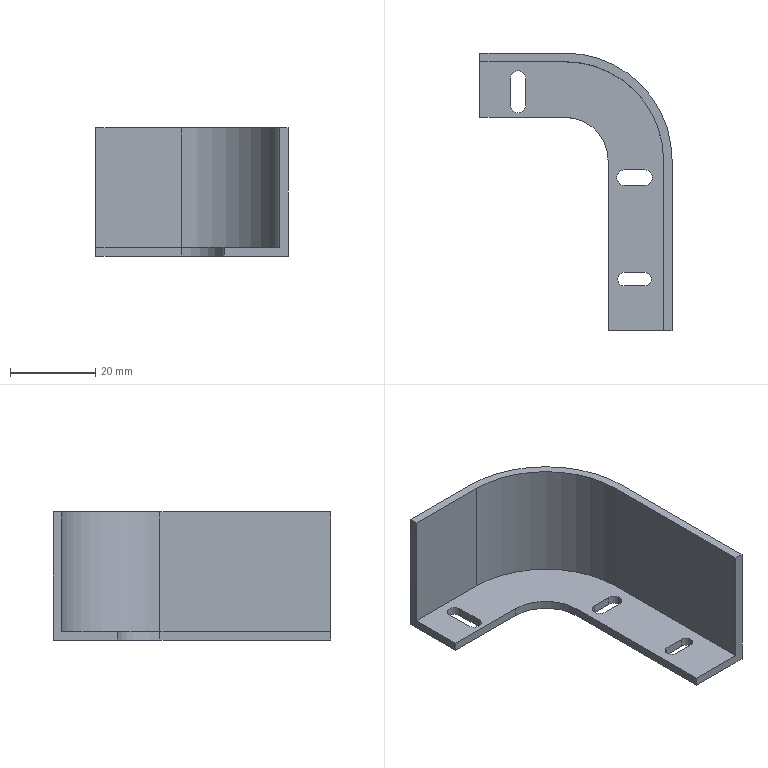Part | SolidWorks | features ICE 2, ExtruThin 1 | 1 solid | 28 faces | box 45 x 65 x 30 mm | volume 7932 mm3 | plane 17 | cylinder 11 | commonest cylinder face diameters 3.152 x3 3.6 x3 3.503 x2 20 x1 46 x1 50 x1
STEP:
#1=CARTESIAN_POINT('',(10.165,12.12,0.));
#2=VERTEX_POINT('',#1);
#3=CARTESIAN_POINT('',(8.588,13.696,0.));
#4=VERTEX_POINT('',#3);
#5=CARTESIAN_POINT('',(8.588,12.12,0.));
#6=DIRECTION('',(0.,0.,1.));
#7=DIRECTION('',(1.,0.,0.));
#8=AXIS2_PLACEMENT_3D('',#5,#6,#7);
#9=CIRCLE('',#8,1.576);
#10=EDGE_CURVE('',#2,#4,#9,.T.);
#11=ORIENTED_EDGE('',*,*,#10,.F.);
#12=CARTESIAN_POINT('',(10.165,12.12,2.));
#13=VERTEX_POINT('',#12);
#14=CARTESIAN_POINT('',(10.165,12.12,-26.));
#15=DIRECTION('',(0.,0.,1.));
#16=VECTOR('',#15,1000.);
#17=LINE('',#14,#16);
#18=EDGE_CURVE('',#2,#13,#17,.T.);
#19=ORIENTED_EDGE('',*,*,#18,.T.);
#20=CARTESIAN_POINT('',(8.588,13.696,2.));
#21=VERTEX_POINT('',#20);
#22=CARTESIAN_POINT('',(8.588,12.12,2.));
#23=DIRECTION('',(0.,0.,1.));
#24=DIRECTION('',(1.,0.,0.));
#25=AXIS2_PLACEMENT_3D('',#22,#23,#24);
#26=CIRCLE('',#25,1.576);
#27=EDGE_CURVE('',#13,#21,#26,.T.);
#28=ORIENTED_EDGE('',*,*,#27,.T.);
#29=CARTESIAN_POINT('',(8.588,13.696,-26.));
#30=DIRECTION('',(0.,0.,1.));
#31=VECTOR('',#30,1000.);
#32=LINE('',#29,#31);
#33=EDGE_CURVE('',#4,#21,#32,.T.);
#34=ORIENTED_EDGE('',*,*,#33,.F.);
#35=EDGE_LOOP('',(#11,#19,#28,#34));
#36=FACE_OUTER_BOUND('',#35,.T.);
#37=CARTESIAN_POINT('',(8.588,12.12,-26.));
#38=DIRECTION('',(0.,0.,1.));
#39=DIRECTION('',(1.,0.,0.));
#40=AXIS2_PLACEMENT_3D('',#37,#38,#39);
#41=CYLINDRICAL_SURFACE('',#40,1.576);
#42=ADVANCED_FACE('',(#36),#41,.F.);
#43=CARTESIAN_POINT('',(10.388,35.907,0.));
#44=VERTEX_POINT('',#43);
#45=CARTESIAN_POINT('',(8.588,37.707,0.));
#46=VERTEX_POINT('',#45);
#47=CARTESIAN_POINT('',(8.588,35.907,0.));
#48=DIRECTION('',(0.,0.,1.));
#49=DIRECTION('',(1.,0.,0.));
#50=AXIS2_PLACEMENT_3D('',#47,#48,#49);
#51=CIRCLE('',#50,1.8);
#52=EDGE_CURVE('',#44,#46,#51,.T.);
#53=ORIENTED_EDGE('',*,*,#52,.F.);
#54=CARTESIAN_POINT('',(10.388,35.907,2.));
#55=VERTEX_POINT('',#54);
#56=CARTESIAN_POINT('',(10.388,35.907,-26.));
#57=DIRECTION('',(0.,0.,1.));
#58=VECTOR('',#57,1000.);
#59=LINE('',#56,#58);
#60=EDGE_CURVE('',#44,#55,#59,.T.);
#61=ORIENTED_EDGE('',*,*,#60,.T.);
#62=CARTESIAN_POINT('',(8.588,37.707,2.));
#63=VERTEX_POINT('',#62);
#64=CARTESIAN_POINT('',(8.588,35.907,2.));
#65=DIRECTION('',(0.,0.,1.));
#66=DIRECTION('',(1.,0.,0.));
#67=AXIS2_PLACEMENT_3D('',#64,#65,#66);
#68=CIRCLE('',#67,1.8);
#69=EDGE_CURVE('',#55,#63,#68,.T.);
#70=ORIENTED_EDGE('',*,*,#69,.T.);
#71=CARTESIAN_POINT('',(8.588,37.707,-26.));
#72=DIRECTION('',(0.,0.,1.));
#73=VECTOR('',#72,1000.);
#74=LINE('',#71,#73);
#75=EDGE_CURVE('',#46,#63,#74,.T.);
#76=ORIENTED_EDGE('',*,*,#75,.F.);
#77=EDGE_LOOP('',(#53,#61,#70,#76));
#78=FACE_OUTER_BOUND('',#77,.T.);
#79=CARTESIAN_POINT('',(8.588,35.907,-26.));
#80=DIRECTION('',(0.,0.,1.));
#81=DIRECTION('',(1.,0.,0.));
#82=AXIS2_PLACEMENT_3D('',#79,#80,#81);
#83=CYLINDRICAL_SURFACE('',#82,1.8);
#84=ADVANCED_FACE('',(#78),#83,.F.);
#85=CARTESIAN_POINT('',(-10.,65.,0.));
#86=VERTEX_POINT('',#85);
#87=CARTESIAN_POINT('',(-30.,65.,0.));
#88=VERTEX_POINT('',#87);
#89=CARTESIAN_POINT('',(-10.,65.,0.));
#90=DIRECTION('',(-1.,0.,0.));
#91=VECTOR('',#90,1000.);
#92=LINE('',#89,#91);
#93=EDGE_CURVE('',#86,#88,#92,.T.);
#94=ORIENTED_EDGE('',*,*,#93,.T.);
#95=CARTESIAN_POINT('',(-30.,65.,30.));
#96=VERTEX_POINT('',#95);
#97=CARTESIAN_POINT('',(-30.,65.,2.));
#98=DIRECTION('',(0.,0.,-1.));
#99=VECTOR('',#98,1000.);
#100=LINE('',#97,#99);
#101=EDGE_CURVE('',#96,#88,#100,.T.);
#102=ORIENTED_EDGE('',*,*,#101,.F.);
#103=CARTESIAN_POINT('',(-10.,65.,30.));
#104=VERTEX_POINT('',#103);
#105=CARTESIAN_POINT('',(-10.,65.,30.));
#106=DIRECTION('',(-1.,0.,0.));
#107=VECTOR('',#106,1000.);
#108=LINE('',#105,#107);
#109=EDGE_CURVE('',#104,#96,#108,.T.);
#110=ORIENTED_EDGE('',*,*,#109,.F.);
#111=CARTESIAN_POINT('',(-10.,65.,2.));
#112=DIRECTION('',(0.,0.,-1.));
#113=VECTOR('',#112,1000.);
#114=LINE('',#111,#113);
#115=EDGE_CURVE('',#104,#86,#114,.T.);
#116=ORIENTED_EDGE('',*,*,#115,.T.);
#117=EDGE_LOOP('',(#94,#102,#110,#116));
#118=FACE_OUTER_BOUND('',#117,.T.);
#119=CARTESIAN_POINT('',(-10.,65.,2.));
#120=DIRECTION('',(0.,-1.,0.));
#121=DIRECTION('',(1.,0.,0.));
#122=AXIS2_PLACEMENT_3D('',#119,#120,#121);
#123=PLANE('',#122);
#124=ADVANCED_FACE('',(#118),#123,.F.);
#125=CARTESIAN_POINT('',(-30.,50.,0.));
#126=VERTEX_POINT('',#125);
#127=CARTESIAN_POINT('',(-30.,50.,0.));
#128=DIRECTION('',(0.,1.,0.));
#129=VECTOR('',#128,1000.);
#130=LINE('',#127,#129);
#131=EDGE_CURVE('',#126,#88,#130,.T.);
#132=ORIENTED_EDGE('',*,*,#131,.F.);
#133=CARTESIAN_POINT('',(-30.,50.,2.));
#134=VERTEX_POINT('',#133);
#135=CARTESIAN_POINT('',(-30.,50.,2.));
#136=DIRECTION('',(0.,0.,-1.));
#137=VECTOR('',#136,1000.);
#138=LINE('',#135,#137);
#139=EDGE_CURVE('',#134,#126,#138,.T.);
#140=ORIENTED_EDGE('',*,*,#139,.F.);
#141=CARTESIAN_POINT('',(-30.,63.,2.));
#142=VERTEX_POINT('',#141);
#143=CARTESIAN_POINT('',(-30.,50.,2.));
#144=DIRECTION('',(0.,1.,0.));
#145=VECTOR('',#144,1000.);
#146=LINE('',#143,#145);
#147=EDGE_CURVE('',#134,#142,#146,.T.);
#148=ORIENTED_EDGE('',*,*,#147,.T.);
#149=CARTESIAN_POINT('',(-30.,63.,30.));
#150=VERTEX_POINT('',#149);
#151=CARTESIAN_POINT('',(-30.,63.,30.));
#152=DIRECTION('',(0.,0.,-1.));
#153=VECTOR('',#152,1000.);
#154=LINE('',#151,#153);
#155=EDGE_CURVE('',#150,#142,#154,.T.);
#156=ORIENTED_EDGE('',*,*,#155,.F.);
#157=CARTESIAN_POINT('',(-30.,65.,30.));
#158=DIRECTION('',(0.,-1.,0.));
#159=VECTOR('',#158,1000.);
#160=LINE('',#157,#159);
#161=EDGE_CURVE('',#96,#150,#160,.T.);
#162=ORIENTED_EDGE('',*,*,#161,.F.);
#163=ORIENTED_EDGE('',*,*,#101,.T.);
#164=EDGE_LOOP('',(#132,#140,#148,#156,#162,#163));
#165=FACE_OUTER_BOUND('',#164,.T.);
#166=CARTESIAN_POINT('',(-30.,50.,2.));
#167=DIRECTION('',(-1.,0.,0.));
#168=DIRECTION('',(0.,-1.,0.));
#169=AXIS2_PLACEMENT_3D('',#166,#167,#168);
#170=PLANE('',#169);
#171=ADVANCED_FACE('',(#165),#170,.T.);
#172=CARTESIAN_POINT('',(-10.,50.,0.));
#173=VERTEX_POINT('',#172);
#174=CARTESIAN_POINT('',(-10.,50.,0.));
#175=DIRECTION('',(-1.,0.,0.));
#176=VECTOR('',#175,1000.);
#177=LINE('',#174,#176);
#178=EDGE_CURVE('',#173,#126,#177,.T.);
#179=ORIENTED_EDGE('',*,*,#178,.F.);
#180=CARTESIAN_POINT('',(-10.,50.,2.));
#181=VERTEX_POINT('',#180);
#182=CARTESIAN_POINT('',(-10.,50.,2.));
#183=DIRECTION('',(0.,0.,-1.));
#184=VECTOR('',#183,1000.);
#185=LINE('',#182,#184);
#186=EDGE_CURVE('',#181,#173,#185,.T.);
#187=ORIENTED_EDGE('',*,*,#186,.F.);
#188=CARTESIAN_POINT('',(-10.,50.,2.));
#189=DIRECTION('',(-1.,0.,0.));
#190=VECTOR('',#189,1000.);
#191=LINE('',#188,#190);
#192=EDGE_CURVE('',#181,#134,#191,.T.);
#193=ORIENTED_EDGE('',*,*,#192,.T.);
#194=ORIENTED_EDGE('',*,*,#139,.T.);
#195=EDGE_LOOP('',(#179,#187,#193,#194));
#196=FACE_OUTER_BOUND('',#195,.T.);
#197=CARTESIAN_POINT('',(-10.,50.,2.));
#198=DIRECTION('',(0.,-1.,0.));
#199=DIRECTION('',(1.,0.,0.));
#200=AXIS2_PLACEMENT_3D('',#197,#198,#199);
#201=PLANE('',#200);
#202=ADVANCED_FACE('',(#196),#201,.T.);
#203=CARTESIAN_POINT('',(0.,40.,0.));
#204=VERTEX_POINT('',#203);
#205=CARTESIAN_POINT('',(-10.,40.,0.));
#206=DIRECTION('',(0.,0.,1.));
#207=DIRECTION('',(1.,0.,0.));
#208=AXIS2_PLACEMENT_3D('',#205,#206,#207);
#209=CIRCLE('',#208,10.);
#210=EDGE_CURVE('',#204,#173,#209,.T.);
#211=ORIENTED_EDGE('',*,*,#210,.F.);
#212=CARTESIAN_POINT('',(0.,40.,2.));
#213=VERTEX_POINT('',#212);
#214=CARTESIAN_POINT('',(0.,40.,2.));
#215=DIRECTION('',(0.,0.,-1.));
#216=VECTOR('',#215,1000.);
#217=LINE('',#214,#216);
#218=EDGE_CURVE('',#213,#204,#217,.T.);
#219=ORIENTED_EDGE('',*,*,#218,.F.);
#220=CARTESIAN_POINT('',(-10.,40.,2.));
#221=DIRECTION('',(0.,0.,1.));
#222=DIRECTION('',(1.,0.,0.));
#223=AXIS2_PLACEMENT_3D('',#220,#221,#222);
#224=CIRCLE('',#223,10.);
#225=EDGE_CURVE('',#213,#181,#224,.T.);
#226=ORIENTED_EDGE('',*,*,#225,.T.);
#227=ORIENTED_EDGE('',*,*,#186,.T.);
#228=EDGE_LOOP('',(#211,#219,#226,#227));
#229=FACE_OUTER_BOUND('',#228,.T.);
#230=CARTESIAN_POINT('',(-10.,40.,2.));
#231=DIRECTION('',(0.,0.,-1.));
#232=DIRECTION('',(-1.,0.,0.));
#233=AXIS2_PLACEMENT_3D('',#230,#231,#232);
#234=CYLINDRICAL_SURFACE('',#233,10.);
#235=ADVANCED_FACE('',(#229),#234,.F.);
#236=CARTESIAN_POINT('',(0.,0.,0.));
#237=VERTEX_POINT('',#236);
#238=CARTESIAN_POINT('',(0.,0.,0.));
#239=DIRECTION('',(0.,1.,0.));
#240=VECTOR('',#239,1000.);
#241=LINE('',#238,#240);
#242=EDGE_CURVE('',#237,#204,#241,.T.);
#243=ORIENTED_EDGE('',*,*,#242,.F.);
#244=CARTESIAN_POINT('',(0.,0.,2.));
#245=VERTEX_POINT('',#244);
#246=CARTESIAN_POINT('',(0.,0.,2.));
#247=DIRECTION('',(0.,0.,-1.));
#248=VECTOR('',#247,1000.);
#249=LINE('',#246,#248);
#250=EDGE_CURVE('',#245,#237,#249,.T.);
#251=ORIENTED_EDGE('',*,*,#250,.F.);
#252=CARTESIAN_POINT('',(0.,0.,2.));
#253=DIRECTION('',(0.,1.,0.));
#254=VECTOR('',#253,1000.);
#255=LINE('',#252,#254);
#256=EDGE_CURVE('',#245,#213,#255,.T.);
#257=ORIENTED_EDGE('',*,*,#256,.T.);
#258=ORIENTED_EDGE('',*,*,#218,.T.);
#259=EDGE_LOOP('',(#243,#251,#257,#258));
#260=FACE_OUTER_BOUND('',#259,.T.);
#261=CARTESIAN_POINT('',(0.,0.,2.));
#262=DIRECTION('',(-1.,0.,0.));
#263=DIRECTION('',(0.,0.,1.));
#264=AXIS2_PLACEMENT_3D('',#261,#262,#263);
#265=PLANE('',#264);
#266=ADVANCED_FACE('',(#260),#265,.T.);
#267=CARTESIAN_POINT('',(15.,0.,0.));
#268=VERTEX_POINT('',#267);
#269=CARTESIAN_POINT('',(15.,0.,0.));
#270=DIRECTION('',(-1.,0.,0.));
#271=VECTOR('',#270,1000.);
#272=LINE('',#269,#271);
#273=EDGE_CURVE('',#268,#237,#272,.T.);
#274=ORIENTED_EDGE('',*,*,#273,.F.);
#275=CARTESIAN_POINT('',(15.,0.,30.));
#276=VERTEX_POINT('',#275);
#277=CARTESIAN_POINT('',(15.,0.,2.));
#278=DIRECTION('',(0.,0.,-1.));
#279=VECTOR('',#278,1000.);
#280=LINE('',#277,#279);
#281=EDGE_CURVE('',#276,#268,#280,.T.);
#282=ORIENTED_EDGE('',*,*,#281,.F.);
#283=CARTESIAN_POINT('',(13.,0.,30.));
#284=VERTEX_POINT('',#283);
#285=CARTESIAN_POINT('',(15.,0.,30.));
#286=DIRECTION('',(1.,0.,0.));
#287=VECTOR('',#286,1000.);
#288=LINE('',#285,#287);
#289=EDGE_CURVE('',#284,#276,#288,.T.);
#290=ORIENTED_EDGE('',*,*,#289,.F.);
#291=CARTESIAN_POINT('',(13.,0.,2.));
#292=VERTEX_POINT('',#291);
#293=CARTESIAN_POINT('',(13.,0.,30.));
#294=DIRECTION('',(0.,0.,-1.));
#295=VECTOR('',#294,1000.);
#296=LINE('',#293,#295);
#297=EDGE_CURVE('',#284,#292,#296,.T.);
#298=ORIENTED_EDGE('',*,*,#297,.T.);
#299=CARTESIAN_POINT('',(15.,0.,2.));
#300=DIRECTION('',(-1.,0.,0.));
#301=VECTOR('',#300,1000.);
#302=LINE('',#299,#301);
#303=EDGE_CURVE('',#292,#245,#302,.T.);
#304=ORIENTED_EDGE('',*,*,#303,.T.);
#305=ORIENTED_EDGE('',*,*,#250,.T.);
#306=EDGE_LOOP('',(#274,#282,#290,#298,#304,#305));
#307=FACE_OUTER_BOUND('',#306,.T.);
#308=CARTESIAN_POINT('',(15.,0.,2.));
#309=DIRECTION('',(0.,-1.,0.));
#310=DIRECTION('',(0.,0.,-1.));
#311=AXIS2_PLACEMENT_3D('',#308,#309,#310);
#312=PLANE('',#311);
#313=ADVANCED_FACE('',(#307),#312,.T.);
#314=CARTESIAN_POINT('',(15.,40.,0.));
#315=VERTEX_POINT('',#314);
#316=CARTESIAN_POINT('',(15.,0.,0.));
#317=DIRECTION('',(0.,1.,0.));
#318=VECTOR('',#317,1000.);
#319=LINE('',#316,#318);
#320=EDGE_CURVE('',#268,#315,#319,.T.);
#321=ORIENTED_EDGE('',*,*,#320,.T.);
#322=CARTESIAN_POINT('',(15.,40.,30.));
#323=VERTEX_POINT('',#322);
#324=CARTESIAN_POINT('',(15.,40.,2.));
#325=DIRECTION('',(0.,0.,-1.));
#326=VECTOR('',#325,1000.);
#327=LINE('',#324,#326);
#328=EDGE_CURVE('',#323,#315,#327,.T.);
#329=ORIENTED_EDGE('',*,*,#328,.F.);
#330=CARTESIAN_POINT('',(15.,0.,30.));
#331=DIRECTION('',(0.,1.,0.));
#332=VECTOR('',#331,1000.);
#333=LINE('',#330,#332);
#334=EDGE_CURVE('',#276,#323,#333,.T.);
#335=ORIENTED_EDGE('',*,*,#334,.F.);
#336=ORIENTED_EDGE('',*,*,#281,.T.);
#337=EDGE_LOOP('',(#321,#329,#335,#336));
#338=FACE_OUTER_BOUND('',#337,.T.);
#339=CARTESIAN_POINT('',(15.,0.,2.));
#340=DIRECTION('',(-1.,0.,0.));
#341=DIRECTION('',(0.,0.,1.));
#342=AXIS2_PLACEMENT_3D('',#339,#340,#341);
#343=PLANE('',#342);
#344=ADVANCED_FACE('',(#338),#343,.F.);
#345=CARTESIAN_POINT('',(-10.,40.,0.));
#346=DIRECTION('',(0.,0.,1.));
#347=DIRECTION('',(1.,0.,0.));
#348=AXIS2_PLACEMENT_3D('',#345,#346,#347);
#349=CIRCLE('',#348,25.);
#350=EDGE_CURVE('',#315,#86,#349,.T.);
#351=ORIENTED_EDGE('',*,*,#350,.T.);
#352=ORIENTED_EDGE('',*,*,#115,.F.);
#353=CARTESIAN_POINT('',(-10.,40.,30.));
#354=DIRECTION('',(0.,0.,1.));
#355=DIRECTION('',(1.,0.,0.));
#356=AXIS2_PLACEMENT_3D('',#353,#354,#355);
#357=CIRCLE('',#356,25.);
#358=EDGE_CURVE('',#323,#104,#357,.T.);
#359=ORIENTED_EDGE('',*,*,#358,.F.);
#360=ORIENTED_EDGE('',*,*,#328,.T.);
#361=EDGE_LOOP('',(#351,#352,#359,#360));
#362=FACE_OUTER_BOUND('',#361,.T.);
#363=CARTESIAN_POINT('',(-10.,40.,2.));
#364=DIRECTION('',(0.,0.,-1.));
#365=DIRECTION('',(-1.,0.,0.));
#366=AXIS2_PLACEMENT_3D('',#363,#364,#365);
#367=CYLINDRICAL_SURFACE('',#366,25.);
#368=ADVANCED_FACE('',(#362),#367,.T.);
#369=CARTESIAN_POINT('',(3.842,13.696,2.));
#370=VERTEX_POINT('',#369);
#371=CARTESIAN_POINT('',(3.842,10.543,2.));
#372=VERTEX_POINT('',#371);
#373=CARTESIAN_POINT('',(3.842,12.12,2.));
#374=DIRECTION('',(0.,0.,1.));
#375=DIRECTION('',(1.,0.,0.));
#376=AXIS2_PLACEMENT_3D('',#373,#374,#375);
#377=CIRCLE('',#376,1.576);
#378=EDGE_CURVE('',#370,#372,#377,.T.);
#379=ORIENTED_EDGE('',*,*,#378,.F.);
#380=CARTESIAN_POINT('',(3.842,13.696,2.));
#381=DIRECTION('',(-1.,0.,0.));
#382=VECTOR('',#381,1000.);
#383=LINE('',#380,#382);
#384=EDGE_CURVE('',#21,#370,#383,.T.);
#385=ORIENTED_EDGE('',*,*,#384,.F.);
#386=ORIENTED_EDGE('',*,*,#27,.F.);
#387=CARTESIAN_POINT('',(8.588,10.543,2.));
#388=VERTEX_POINT('',#387);
#389=CARTESIAN_POINT('',(8.588,12.12,2.));
#390=DIRECTION('',(0.,0.,1.));
#391=DIRECTION('',(1.,0.,0.));
#392=AXIS2_PLACEMENT_3D('',#389,#390,#391);
#393=CIRCLE('',#392,1.576);
#394=EDGE_CURVE('',#388,#13,#393,.T.);
#395=ORIENTED_EDGE('',*,*,#394,.F.);
#396=CARTESIAN_POINT('',(3.842,10.543,2.));
#397=DIRECTION('',(1.,0.,0.));
#398=VECTOR('',#397,1000.);
#399=LINE('',#396,#398);
#400=EDGE_CURVE('',#372,#388,#399,.T.);
#401=ORIENTED_EDGE('',*,*,#400,.F.);
#402=EDGE_LOOP('',(#379,#385,#386,#395,#401));
#403=FACE_BOUND('',#402,.T.);
#404=CARTESIAN_POINT('',(3.842,37.707,2.));
#405=VERTEX_POINT('',#404);
#406=CARTESIAN_POINT('',(3.842,34.107,2.));
#407=VERTEX_POINT('',#406);
#408=CARTESIAN_POINT('',(3.842,35.907,2.));
#409=DIRECTION('',(0.,0.,1.));
#410=DIRECTION('',(1.,0.,0.));
#411=AXIS2_PLACEMENT_3D('',#408,#409,#410);
#412=CIRCLE('',#411,1.8);
#413=EDGE_CURVE('',#405,#407,#412,.T.);
#414=ORIENTED_EDGE('',*,*,#413,.F.);
#415=CARTESIAN_POINT('',(3.842,37.707,2.));
#416=DIRECTION('',(-1.,0.,0.));
#417=VECTOR('',#416,1000.);
#418=LINE('',#415,#417);
#419=EDGE_CURVE('',#63,#405,#418,.T.);
#420=ORIENTED_EDGE('',*,*,#419,.F.);
#421=ORIENTED_EDGE('',*,*,#69,.F.);
#422=CARTESIAN_POINT('',(8.588,34.107,2.));
#423=VERTEX_POINT('',#422);
#424=CARTESIAN_POINT('',(8.588,35.907,2.));
#425=DIRECTION('',(0.,0.,1.));
#426=DIRECTION('',(1.,0.,0.));
#427=AXIS2_PLACEMENT_3D('',#424,#425,#426);
#428=CIRCLE('',#427,1.8);
#429=EDGE_CURVE('',#423,#55,#428,.T.);
#430=ORIENTED_EDGE('',*,*,#429,.F.);
#431=CARTESIAN_POINT('',(3.842,34.107,2.));
#432=DIRECTION('',(1.,0.,0.));
#433=VECTOR('',#432,1000.);
#434=LINE('',#431,#433);
#435=EDGE_CURVE('',#407,#423,#434,.T.);
#436=ORIENTED_EDGE('',*,*,#435,.F.);
#437=EDGE_LOOP('',(#414,#420,#421,#430,#436));
#438=FACE_BOUND('',#437,.T.);
#439=CARTESIAN_POINT('',(-19.284,59.176,2.));
#440=VERTEX_POINT('',#439);
#441=CARTESIAN_POINT('',(-22.787,59.176,2.));
#442=VERTEX_POINT('',#441);
#443=CARTESIAN_POINT('',(-21.035,59.176,2.));
#444=DIRECTION('',(0.,0.,1.));
#445=DIRECTION('',(1.,0.,0.));
#446=AXIS2_PLACEMENT_3D('',#443,#444,#445);
#447=CIRCLE('',#446,1.751);
#448=EDGE_CURVE('',#440,#442,#447,.T.);
#449=ORIENTED_EDGE('',*,*,#448,.F.);
#450=CARTESIAN_POINT('',(-19.284,52.836,2.));
#451=VERTEX_POINT('',#450);
#452=CARTESIAN_POINT('',(-19.284,59.176,2.));
#453=DIRECTION('',(0.,1.,0.));
#454=VECTOR('',#453,1000.);
#455=LINE('',#452,#454);
#456=EDGE_CURVE('',#451,#440,#455,.T.);
#457=ORIENTED_EDGE('',*,*,#456,.F.);
#458=CARTESIAN_POINT('',(-22.787,52.836,2.));
#459=VERTEX_POINT('',#458);
#460=CARTESIAN_POINT('',(-21.035,52.836,2.));
#461=DIRECTION('',(0.,0.,1.));
#462=DIRECTION('',(1.,0.,0.));
#463=AXIS2_PLACEMENT_3D('',#460,#461,#462);
#464=CIRCLE('',#463,1.751);
#465=EDGE_CURVE('',#459,#451,#464,.T.);
#466=ORIENTED_EDGE('',*,*,#465,.F.);
#467=CARTESIAN_POINT('',(-22.787,59.176,2.));
#468=DIRECTION('',(0.,-1.,0.));
#469=VECTOR('',#468,1000.);
#470=LINE('',#467,#469);
#471=EDGE_CURVE('',#442,#459,#470,.T.);
#472=ORIENTED_EDGE('',*,*,#471,.F.);
#473=EDGE_LOOP('',(#449,#457,#466,#472));
#474=FACE_BOUND('',#473,.T.);
#475=CARTESIAN_POINT('',(13.,40.,2.));
#476=VERTEX_POINT('',#475);
#477=CARTESIAN_POINT('',(13.,0.,2.));
#478=DIRECTION('',(0.,-1.,0.));
#479=VECTOR('',#478,1000.);
#480=LINE('',#477,#479);
#481=EDGE_CURVE('',#476,#292,#480,.T.);
#482=ORIENTED_EDGE('',*,*,#481,.F.);
#483=CARTESIAN_POINT('',(-10.,63.,2.));
#484=VERTEX_POINT('',#483);
#485=CARTESIAN_POINT('',(-10.,40.,2.));
#486=DIRECTION('',(0.,0.,-1.));
#487=DIRECTION('',(1.,0.,0.));
#488=AXIS2_PLACEMENT_3D('',#485,#486,#487);
#489=CIRCLE('',#488,23.);
#490=EDGE_CURVE('',#484,#476,#489,.T.);
#491=ORIENTED_EDGE('',*,*,#490,.F.);
#492=CARTESIAN_POINT('',(-10.,63.,2.));
#493=DIRECTION('',(1.,0.,0.));
#494=VECTOR('',#493,1000.);
#495=LINE('',#492,#494);
#496=EDGE_CURVE('',#142,#484,#495,.T.);
#497=ORIENTED_EDGE('',*,*,#496,.F.);
#498=ORIENTED_EDGE('',*,*,#147,.F.);
#499=ORIENTED_EDGE('',*,*,#192,.F.);
#500=ORIENTED_EDGE('',*,*,#225,.F.);
#501=ORIENTED_EDGE('',*,*,#256,.F.);
#502=ORIENTED_EDGE('',*,*,#303,.F.);
#503=EDGE_LOOP('',(#482,#491,#497,#498,#499,#500,#501,#502));
#504=FACE_OUTER_BOUND('',#503,.T.);
#505=CARTESIAN_POINT('',(-10.,40.,2.));
#506=DIRECTION('',(0.,0.,1.));
#507=DIRECTION('',(1.,0.,0.));
#508=AXIS2_PLACEMENT_3D('',#505,#506,#507);
#509=PLANE('',#508);
#510=ADVANCED_FACE('',(#403,#438,#474,#504),#509,.T.);
#511=CARTESIAN_POINT('',(3.842,13.696,0.));
#512=VERTEX_POINT('',#511);
#513=CARTESIAN_POINT('',(-10.,13.696,0.));
#514=DIRECTION('',(-1.,0.,0.));
#515=VECTOR('',#514,1000.);
#516=LINE('',#513,#515);
#517=EDGE_CURVE('',#4,#512,#516,.T.);
#518=ORIENTED_EDGE('',*,*,#517,.T.);
#519=CARTESIAN_POINT('',(3.842,10.543,0.));
#520=VERTEX_POINT('',#519);
#521=CARTESIAN_POINT('',(3.842,12.12,0.));
#522=DIRECTION('',(0.,0.,1.));
#523=DIRECTION('',(1.,0.,0.));
#524=AXIS2_PLACEMENT_3D('',#521,#522,#523);
#525=CIRCLE('',#524,1.576);
#526=EDGE_CURVE('',#512,#520,#525,.T.);
#527=ORIENTED_EDGE('',*,*,#526,.T.);
#528=CARTESIAN_POINT('',(8.588,10.543,0.));
#529=VERTEX_POINT('',#528);
#530=CARTESIAN_POINT('',(-10.,10.543,0.));
#531=DIRECTION('',(1.,0.,0.));
#532=VECTOR('',#531,1000.);
#533=LINE('',#530,#532);
#534=EDGE_CURVE('',#520,#529,#533,.T.);
#535=ORIENTED_EDGE('',*,*,#534,.T.);
#536=CARTESIAN_POINT('',(8.588,12.12,0.));
#537=DIRECTION('',(0.,0.,1.));
#538=DIRECTION('',(1.,0.,0.));
#539=AXIS2_PLACEMENT_3D('',#536,#537,#538);
#540=CIRCLE('',#539,1.576);
#541=EDGE_CURVE('',#529,#2,#540,.T.);
#542=ORIENTED_EDGE('',*,*,#541,.T.);
#543=ORIENTED_EDGE('',*,*,#10,.T.);
#544=EDGE_LOOP('',(#518,#527,#535,#542,#543));
#545=FACE_BOUND('',#544,.T.);
#546=CARTESIAN_POINT('',(3.842,37.707,0.));
#547=VERTEX_POINT('',#546);
#548=CARTESIAN_POINT('',(-10.,37.707,0.));
#549=DIRECTION('',(-1.,0.,0.));
#550=VECTOR('',#549,1000.);
#551=LINE('',#548,#550);
#552=EDGE_CURVE('',#46,#547,#551,.T.);
#553=ORIENTED_EDGE('',*,*,#552,.T.);
#554=CARTESIAN_POINT('',(3.842,34.107,0.));
#555=VERTEX_POINT('',#554);
#556=CARTESIAN_POINT('',(3.842,35.907,0.));
#557=DIRECTION('',(0.,0.,1.));
#558=DIRECTION('',(1.,0.,0.));
#559=AXIS2_PLACEMENT_3D('',#556,#557,#558);
#560=CIRCLE('',#559,1.8);
#561=EDGE_CURVE('',#547,#555,#560,.T.);
#562=ORIENTED_EDGE('',*,*,#561,.T.);
#563=CARTESIAN_POINT('',(8.588,34.107,0.));
#564=VERTEX_POINT('',#563);
#565=CARTESIAN_POINT('',(-10.,34.107,0.));
#566=DIRECTION('',(1.,0.,0.));
#567=VECTOR('',#566,1000.);
#568=LINE('',#565,#567);
#569=EDGE_CURVE('',#555,#564,#568,.T.);
#570=ORIENTED_EDGE('',*,*,#569,.T.);
#571=CARTESIAN_POINT('',(8.588,35.907,0.));
#572=DIRECTION('',(0.,0.,1.));
#573=DIRECTION('',(1.,0.,0.));
#574=AXIS2_PLACEMENT_3D('',#571,#572,#573);
#575=CIRCLE('',#574,1.8);
#576=EDGE_CURVE('',#564,#44,#575,.T.);
#577=ORIENTED_EDGE('',*,*,#576,.T.);
#578=ORIENTED_EDGE('',*,*,#52,.T.);
#579=EDGE_LOOP('',(#553,#562,#570,#577,#578));
#580=FACE_BOUND('',#579,.T.);
#581=CARTESIAN_POINT('',(-19.284,52.836,0.));
#582=VERTEX_POINT('',#581);
#583=CARTESIAN_POINT('',(-19.284,59.176,0.));
#584=VERTEX_POINT('',#583);
#585=CARTESIAN_POINT('',(-19.284,40.,0.));
#586=DIRECTION('',(0.,1.,0.));
#587=VECTOR('',#586,1000.);
#588=LINE('',#585,#587);
#589=EDGE_CURVE('',#582,#584,#588,.T.);
#590=ORIENTED_EDGE('',*,*,#589,.T.);
#591=CARTESIAN_POINT('',(-22.787,59.176,0.));
#592=VERTEX_POINT('',#591);
#593=CARTESIAN_POINT('',(-21.035,59.176,0.));
#594=DIRECTION('',(0.,0.,1.));
#595=DIRECTION('',(1.,0.,0.));
#596=AXIS2_PLACEMENT_3D('',#593,#594,#595);
#597=CIRCLE('',#596,1.751);
#598=EDGE_CURVE('',#584,#592,#597,.T.);
#599=ORIENTED_EDGE('',*,*,#598,.T.);
#600=CARTESIAN_POINT('',(-22.787,52.836,0.));
#601=VERTEX_POINT('',#600);
#602=CARTESIAN_POINT('',(-22.787,40.,0.));
#603=DIRECTION('',(0.,-1.,0.));
#604=VECTOR('',#603,1000.);
#605=LINE('',#602,#604);
#606=EDGE_CURVE('',#592,#601,#605,.T.);
#607=ORIENTED_EDGE('',*,*,#606,.T.);
#608=CARTESIAN_POINT('',(-21.035,52.836,0.));
#609=DIRECTION('',(0.,0.,1.));
#610=DIRECTION('',(1.,0.,0.));
#611=AXIS2_PLACEMENT_3D('',#608,#609,#610);
#612=CIRCLE('',#611,1.751);
#613=EDGE_CURVE('',#601,#582,#612,.T.);
#614=ORIENTED_EDGE('',*,*,#613,.T.);
#615=EDGE_LOOP('',(#590,#599,#607,#614));
#616=FACE_BOUND('',#615,.T.);
#617=ORIENTED_EDGE('',*,*,#93,.F.);
#618=ORIENTED_EDGE('',*,*,#350,.F.);
#619=ORIENTED_EDGE('',*,*,#320,.F.);
#620=ORIENTED_EDGE('',*,*,#273,.T.);
#621=ORIENTED_EDGE('',*,*,#242,.T.);
#622=ORIENTED_EDGE('',*,*,#210,.T.);
#623=ORIENTED_EDGE('',*,*,#178,.T.);
#624=ORIENTED_EDGE('',*,*,#131,.T.);
#625=EDGE_LOOP('',(#617,#618,#619,#620,#621,#622,#623,#624));
#626=FACE_OUTER_BOUND('',#625,.T.);
#627=CARTESIAN_POINT('',(-10.,40.,0.));
#628=DIRECTION('',(0.,0.,1.));
#629=DIRECTION('',(1.,0.,0.));
#630=AXIS2_PLACEMENT_3D('',#627,#628,#629);
#631=PLANE('',#630);
#632=ADVANCED_FACE('',(#545,#580,#616,#626),#631,.F.);
#633=ORIENTED_EDGE('',*,*,#496,.T.);
#634=CARTESIAN_POINT('',(-10.,63.,30.));
#635=VERTEX_POINT('',#634);
#636=CARTESIAN_POINT('',(-10.,63.,30.));
#637=DIRECTION('',(0.,0.,-1.));
#638=VECTOR('',#637,1000.);
#639=LINE('',#636,#638);
#640=EDGE_CURVE('',#635,#484,#639,.T.);
#641=ORIENTED_EDGE('',*,*,#640,.F.);
#642=CARTESIAN_POINT('',(-10.,63.,30.));
#643=DIRECTION('',(1.,0.,0.));
#644=VECTOR('',#643,1000.);
#645=LINE('',#642,#644);
#646=EDGE_CURVE('',#150,#635,#645,.T.);
#647=ORIENTED_EDGE('',*,*,#646,.F.);
#648=ORIENTED_EDGE('',*,*,#155,.T.);
#649=EDGE_LOOP('',(#633,#641,#647,#648));
#650=FACE_OUTER_BOUND('',#649,.T.);
#651=CARTESIAN_POINT('',(-10.,63.,30.));
#652=DIRECTION('',(0.,1.,0.));
#653=DIRECTION('',(0.,0.,1.));
#654=AXIS2_PLACEMENT_3D('',#651,#652,#653);
#655=PLANE('',#654);
#656=ADVANCED_FACE('',(#650),#655,.F.);
#657=ORIENTED_EDGE('',*,*,#490,.T.);
#658=CARTESIAN_POINT('',(13.,40.,30.));
#659=VERTEX_POINT('',#658);
#660=CARTESIAN_POINT('',(13.,40.,30.));
#661=DIRECTION('',(0.,0.,-1.));
#662=VECTOR('',#661,1000.);
#663=LINE('',#660,#662);
#664=EDGE_CURVE('',#659,#476,#663,.T.);
#665=ORIENTED_EDGE('',*,*,#664,.F.);
#666=CARTESIAN_POINT('',(-10.,40.,30.));
#667=DIRECTION('',(0.,0.,-1.));
#668=DIRECTION('',(1.,0.,0.));
#669=AXIS2_PLACEMENT_3D('',#666,#667,#668);
#670=CIRCLE('',#669,23.);
#671=EDGE_CURVE('',#635,#659,#670,.T.);
#672=ORIENTED_EDGE('',*,*,#671,.F.);
#673=ORIENTED_EDGE('',*,*,#640,.T.);
#674=EDGE_LOOP('',(#657,#665,#672,#673));
#675=FACE_OUTER_BOUND('',#674,.T.);
#676=CARTESIAN_POINT('',(-10.,40.,30.));
#677=DIRECTION('',(0.,0.,-1.));
#678=DIRECTION('',(-1.,0.,0.));
#679=AXIS2_PLACEMENT_3D('',#676,#677,#678);
#680=CYLINDRICAL_SURFACE('',#679,23.);
#681=ADVANCED_FACE('',(#675),#680,.F.);
#682=ORIENTED_EDGE('',*,*,#481,.T.);
#683=ORIENTED_EDGE('',*,*,#297,.F.);
#684=CARTESIAN_POINT('',(13.,0.,30.));
#685=DIRECTION('',(0.,-1.,0.));
#686=VECTOR('',#685,1000.);
#687=LINE('',#684,#686);
#688=EDGE_CURVE('',#659,#284,#687,.T.);
#689=ORIENTED_EDGE('',*,*,#688,.F.);
#690=ORIENTED_EDGE('',*,*,#664,.T.);
#691=EDGE_LOOP('',(#682,#683,#689,#690));
#692=FACE_OUTER_BOUND('',#691,.T.);
#693=CARTESIAN_POINT('',(13.,0.,30.));
#694=DIRECTION('',(1.,0.,0.));
#695=DIRECTION('',(0.,1.,0.));
#696=AXIS2_PLACEMENT_3D('',#693,#694,#695);
#697=PLANE('',#696);
#698=ADVANCED_FACE('',(#692),#697,.F.);
#699=ORIENTED_EDGE('',*,*,#358,.T.);
#700=ORIENTED_EDGE('',*,*,#109,.T.);
#701=ORIENTED_EDGE('',*,*,#161,.T.);
#702=ORIENTED_EDGE('',*,*,#646,.T.);
#703=ORIENTED_EDGE('',*,*,#671,.T.);
#704=ORIENTED_EDGE('',*,*,#688,.T.);
#705=ORIENTED_EDGE('',*,*,#289,.T.);
#706=ORIENTED_EDGE('',*,*,#334,.T.);
#707=EDGE_LOOP('',(#699,#700,#701,#702,#703,#704,#705,#706));
#708=FACE_OUTER_BOUND('',#707,.T.);
#709=CARTESIAN_POINT('',(-10.,40.,30.));
#710=DIRECTION('',(0.,0.,1.));
#711=DIRECTION('',(1.,0.,0.));
#712=AXIS2_PLACEMENT_3D('',#709,#710,#711);
#713=PLANE('',#712);
#714=ADVANCED_FACE('',(#708),#713,.T.);
#715=CARTESIAN_POINT('',(-19.284,59.176,-26.));
#716=DIRECTION('',(0.,0.,1.));
#717=VECTOR('',#716,1000.);
#718=LINE('',#715,#717);
#719=EDGE_CURVE('',#584,#440,#718,.T.);
#720=ORIENTED_EDGE('',*,*,#719,.T.);
#721=ORIENTED_EDGE('',*,*,#448,.T.);
#722=CARTESIAN_POINT('',(-22.787,59.176,-26.));
#723=DIRECTION('',(0.,0.,1.));
#724=VECTOR('',#723,1000.);
#725=LINE('',#722,#724);
#726=EDGE_CURVE('',#592,#442,#725,.T.);
#727=ORIENTED_EDGE('',*,*,#726,.F.);
#728=ORIENTED_EDGE('',*,*,#598,.F.);
#729=EDGE_LOOP('',(#720,#721,#727,#728));
#730=FACE_OUTER_BOUND('',#729,.T.);
#731=CARTESIAN_POINT('',(-21.035,59.176,-26.));
#732=DIRECTION('',(0.,0.,1.));
#733=DIRECTION('',(1.,0.,0.));
#734=AXIS2_PLACEMENT_3D('',#731,#732,#733);
#735=CYLINDRICAL_SURFACE('',#734,1.751);
#736=ADVANCED_FACE('',(#730),#735,.F.);
#737=CARTESIAN_POINT('',(-19.284,52.836,-26.));
#738=DIRECTION('',(0.,0.,1.));
#739=VECTOR('',#738,1000.);
#740=LINE('',#737,#739);
#741=EDGE_CURVE('',#582,#451,#740,.T.);
#742=ORIENTED_EDGE('',*,*,#741,.T.);
#743=ORIENTED_EDGE('',*,*,#456,.T.);
#744=ORIENTED_EDGE('',*,*,#719,.F.);
#745=ORIENTED_EDGE('',*,*,#589,.F.);
#746=EDGE_LOOP('',(#742,#743,#744,#745));
#747=FACE_OUTER_BOUND('',#746,.T.);
#748=CARTESIAN_POINT('',(-19.284,59.176,-26.));
#749=DIRECTION('',(1.,0.,0.));
#750=DIRECTION('',(0.,1.,0.));
#751=AXIS2_PLACEMENT_3D('',#748,#749,#750);
#752=PLANE('',#751);
#753=ADVANCED_FACE('',(#747),#752,.F.);
#754=CARTESIAN_POINT('',(-22.787,52.836,-26.));
#755=DIRECTION('',(0.,0.,1.));
#756=VECTOR('',#755,1000.);
#757=LINE('',#754,#756);
#758=EDGE_CURVE('',#601,#459,#757,.T.);
#759=ORIENTED_EDGE('',*,*,#758,.T.);
#760=ORIENTED_EDGE('',*,*,#465,.T.);
#761=ORIENTED_EDGE('',*,*,#741,.F.);
#762=ORIENTED_EDGE('',*,*,#613,.F.);
#763=EDGE_LOOP('',(#759,#760,#761,#762));
#764=FACE_OUTER_BOUND('',#763,.T.);
#765=CARTESIAN_POINT('',(-21.035,52.836,-26.));
#766=DIRECTION('',(0.,0.,1.));
#767=DIRECTION('',(1.,0.,0.));
#768=AXIS2_PLACEMENT_3D('',#765,#766,#767);
#769=CYLINDRICAL_SURFACE('',#768,1.751);
#770=ADVANCED_FACE('',(#764),#769,.F.);
#771=ORIENTED_EDGE('',*,*,#726,.T.);
#772=ORIENTED_EDGE('',*,*,#471,.T.);
#773=ORIENTED_EDGE('',*,*,#758,.F.);
#774=ORIENTED_EDGE('',*,*,#606,.F.);
#775=EDGE_LOOP('',(#771,#772,#773,#774));
#776=FACE_OUTER_BOUND('',#775,.T.);
#777=CARTESIAN_POINT('',(-22.787,59.176,-26.));
#778=DIRECTION('',(-1.,0.,0.));
#779=DIRECTION('',(0.,-1.,0.));
#780=AXIS2_PLACEMENT_3D('',#777,#778,#779);
#781=PLANE('',#780);
#782=ADVANCED_FACE('',(#776),#781,.F.);
#783=CARTESIAN_POINT('',(3.842,37.707,-26.));
#784=DIRECTION('',(0.,0.,1.));
#785=VECTOR('',#784,1000.);
#786=LINE('',#783,#785);
#787=EDGE_CURVE('',#547,#405,#786,.T.);
#788=ORIENTED_EDGE('',*,*,#787,.T.);
#789=ORIENTED_EDGE('',*,*,#413,.T.);
#790=CARTESIAN_POINT('',(3.842,34.107,-26.));
#791=DIRECTION('',(0.,0.,1.));
#792=VECTOR('',#791,1000.);
#793=LINE('',#790,#792);
#794=EDGE_CURVE('',#555,#407,#793,.T.);
#795=ORIENTED_EDGE('',*,*,#794,.F.);
#796=ORIENTED_EDGE('',*,*,#561,.F.);
#797=EDGE_LOOP('',(#788,#789,#795,#796));
#798=FACE_OUTER_BOUND('',#797,.T.);
#799=CARTESIAN_POINT('',(3.842,35.907,-26.));
#800=DIRECTION('',(0.,0.,1.));
#801=DIRECTION('',(1.,0.,0.));
#802=AXIS2_PLACEMENT_3D('',#799,#800,#801);
#803=CYLINDRICAL_SURFACE('',#802,1.8);
#804=ADVANCED_FACE('',(#798),#803,.F.);
#805=ORIENTED_EDGE('',*,*,#75,.T.);
#806=ORIENTED_EDGE('',*,*,#419,.T.);
#807=ORIENTED_EDGE('',*,*,#787,.F.);
#808=ORIENTED_EDGE('',*,*,#552,.F.);
#809=EDGE_LOOP('',(#805,#806,#807,#808));
#810=FACE_OUTER_BOUND('',#809,.T.);
#811=CARTESIAN_POINT('',(3.842,37.707,-26.));
#812=DIRECTION('',(0.,1.,0.));
#813=DIRECTION('',(0.,0.,1.));
#814=AXIS2_PLACEMENT_3D('',#811,#812,#813);
#815=PLANE('',#814);
#816=ADVANCED_FACE('',(#810),#815,.F.);
#817=ORIENTED_EDGE('',*,*,#60,.F.);
#818=ORIENTED_EDGE('',*,*,#576,.F.);
#819=CARTESIAN_POINT('',(8.588,34.107,-26.));
#820=DIRECTION('',(0.,0.,1.));
#821=VECTOR('',#820,1000.);
#822=LINE('',#819,#821);
#823=EDGE_CURVE('',#564,#423,#822,.T.);
#824=ORIENTED_EDGE('',*,*,#823,.T.);
#825=ORIENTED_EDGE('',*,*,#429,.T.);
#826=EDGE_LOOP('',(#817,#818,#824,#825));
#827=FACE_OUTER_BOUND('',#826,.T.);
#828=CARTESIAN_POINT('',(8.588,35.907,-26.));
#829=DIRECTION('',(0.,0.,1.));
#830=DIRECTION('',(1.,0.,0.));
#831=AXIS2_PLACEMENT_3D('',#828,#829,#830);
#832=CYLINDRICAL_SURFACE('',#831,1.8);
#833=ADVANCED_FACE('',(#827),#832,.F.);
#834=ORIENTED_EDGE('',*,*,#794,.T.);
#835=ORIENTED_EDGE('',*,*,#435,.T.);
#836=ORIENTED_EDGE('',*,*,#823,.F.);
#837=ORIENTED_EDGE('',*,*,#569,.F.);
#838=EDGE_LOOP('',(#834,#835,#836,#837));
#839=FACE_OUTER_BOUND('',#838,.T.);
#840=CARTESIAN_POINT('',(3.842,34.107,-26.));
#841=DIRECTION('',(0.,-1.,0.));
#842=DIRECTION('',(0.,0.,-1.));
#843=AXIS2_PLACEMENT_3D('',#840,#841,#842);
#844=PLANE('',#843);
#845=ADVANCED_FACE('',(#839),#844,.F.);
#846=CARTESIAN_POINT('',(3.842,13.696,-26.));
#847=DIRECTION('',(0.,0.,1.));
#848=VECTOR('',#847,1000.);
#849=LINE('',#846,#848);
#850=EDGE_CURVE('',#512,#370,#849,.T.);
#851=ORIENTED_EDGE('',*,*,#850,.T.);
#852=ORIENTED_EDGE('',*,*,#378,.T.);
#853=CARTESIAN_POINT('',(3.842,10.543,-26.));
#854=DIRECTION('',(0.,0.,1.));
#855=VECTOR('',#854,1000.);
#856=LINE('',#853,#855);
#857=EDGE_CURVE('',#520,#372,#856,.T.);
#858=ORIENTED_EDGE('',*,*,#857,.F.);
#859=ORIENTED_EDGE('',*,*,#526,.F.);
#860=EDGE_LOOP('',(#851,#852,#858,#859));
#861=FACE_OUTER_BOUND('',#860,.T.);
#862=CARTESIAN_POINT('',(3.842,12.12,-26.));
#863=DIRECTION('',(0.,0.,1.));
#864=DIRECTION('',(1.,0.,0.));
#865=AXIS2_PLACEMENT_3D('',#862,#863,#864);
#866=CYLINDRICAL_SURFACE('',#865,1.576);
#867=ADVANCED_FACE('',(#861),#866,.F.);
#868=ORIENTED_EDGE('',*,*,#33,.T.);
#869=ORIENTED_EDGE('',*,*,#384,.T.);
#870=ORIENTED_EDGE('',*,*,#850,.F.);
#871=ORIENTED_EDGE('',*,*,#517,.F.);
#872=EDGE_LOOP('',(#868,#869,#870,#871));
#873=FACE_OUTER_BOUND('',#872,.T.);
#874=CARTESIAN_POINT('',(3.842,13.696,-26.));
#875=DIRECTION('',(0.,1.,0.));
#876=DIRECTION('',(0.,0.,1.));
#877=AXIS2_PLACEMENT_3D('',#874,#875,#876);
#878=PLANE('',#877);
#879=ADVANCED_FACE('',(#873),#878,.F.);
#880=ORIENTED_EDGE('',*,*,#18,.F.);
#881=ORIENTED_EDGE('',*,*,#541,.F.);
#882=CARTESIAN_POINT('',(8.588,10.543,-26.));
#883=DIRECTION('',(0.,0.,1.));
#884=VECTOR('',#883,1000.);
#885=LINE('',#882,#884);
#886=EDGE_CURVE('',#529,#388,#885,.T.);
#887=ORIENTED_EDGE('',*,*,#886,.T.);
#888=ORIENTED_EDGE('',*,*,#394,.T.);
#889=EDGE_LOOP('',(#880,#881,#887,#888));
#890=FACE_OUTER_BOUND('',#889,.T.);
#891=CARTESIAN_POINT('',(8.588,12.12,-26.));
#892=DIRECTION('',(0.,0.,1.));
#893=DIRECTION('',(1.,0.,0.));
#894=AXIS2_PLACEMENT_3D('',#891,#892,#893);
#895=CYLINDRICAL_SURFACE('',#894,1.576);
#896=ADVANCED_FACE('',(#890),#895,.F.);
#897=ORIENTED_EDGE('',*,*,#857,.T.);
#898=ORIENTED_EDGE('',*,*,#400,.T.);
#899=ORIENTED_EDGE('',*,*,#886,.F.);
#900=ORIENTED_EDGE('',*,*,#534,.F.);
#901=EDGE_LOOP('',(#897,#898,#899,#900));
#902=FACE_OUTER_BOUND('',#901,.T.);
#903=CARTESIAN_POINT('',(3.842,10.543,-26.));
#904=DIRECTION('',(0.,-1.,0.));
#905=DIRECTION('',(0.,0.,-1.));
#906=AXIS2_PLACEMENT_3D('',#903,#904,#905);
#907=PLANE('',#906);
#908=ADVANCED_FACE('',(#902),#907,.F.);
#909=CLOSED_SHELL('',(#42,#84,#124,#171,#202,#235,#266,#313,#344,#368,#510,#632,#656,#681,#698,#714,#736,#753,#770,#782,#804,#816,#833,#845,#867,#879,#896,#908));
#910=MANIFOLD_SOLID_BREP('',#909);
#911=CARTESIAN_POINT('',(0.,0.,0.));
#912=DIRECTION('',(0.,0.,1.));
#913=DIRECTION('',(1.,0.,0.));
#914=AXIS2_PLACEMENT_3D('',#911,#912,#913);
#915=(LENGTH_UNIT()NAMED_UNIT(*)SI_UNIT(.MILLI.,.METRE.));
#916=UNCERTAINTY_MEASURE_WITH_UNIT(LENGTH_MEASURE(0.00001),#915,'','');
#917=(NAMED_UNIT(*)PLANE_ANGLE_UNIT()SI_UNIT($,.RADIAN.));
#918=(NAMED_UNIT(*)SI_UNIT($,.STERADIAN.)SOLID_ANGLE_UNIT());
#919=(GEOMETRIC_REPRESENTATION_CONTEXT(3)GLOBAL_UNCERTAINTY_ASSIGNED_CONTEXT((#916))GLOBAL_UNIT_ASSIGNED_CONTEXT((#915,#917,#918))REPRESENTATION_CONTEXT('',''));
#920=ADVANCED_BREP_SHAPE_REPRESENTATION('',(#910,#914),#919);